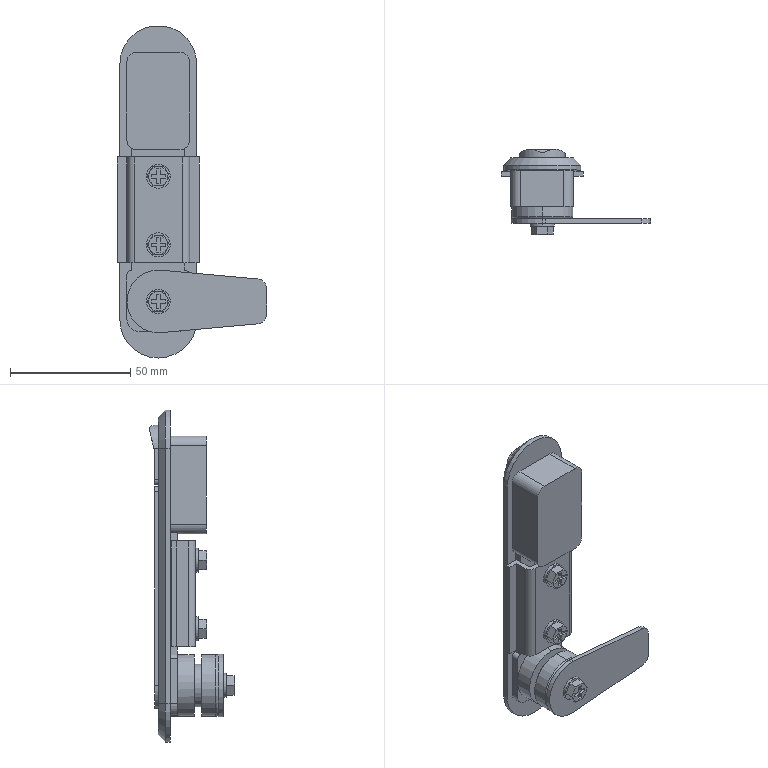Part | NX | features BREP 1 | 1 solid | 191 faces | box 62 x 35.321 x 138 mm | volume 58842 mm3 | plane 121 | cylinder 47 | cone 21 | torus 2 | commonest cylinder face diameters 10 x10 4 x6 8 x6 25.6 x4 19 x3 20 x3